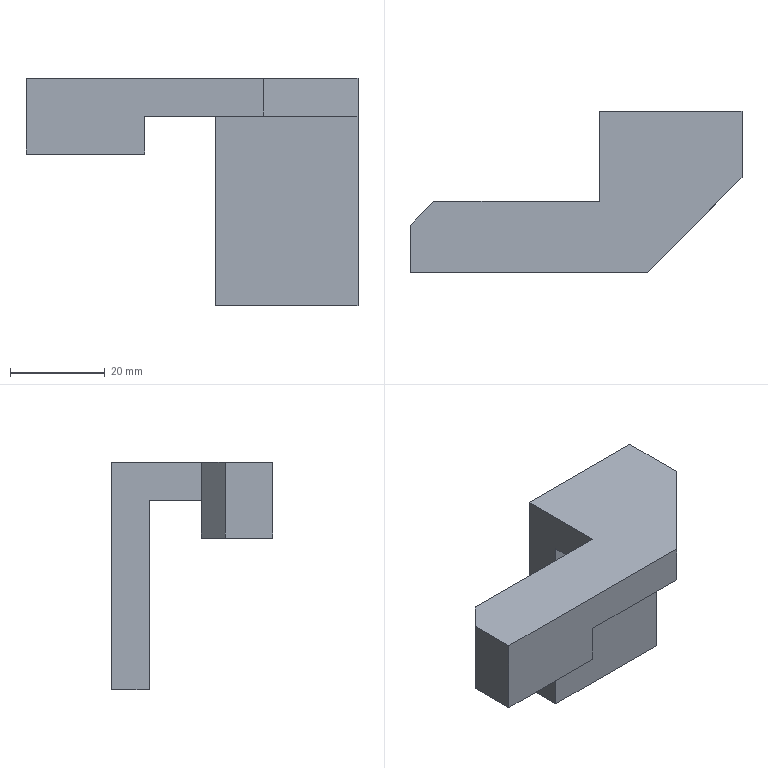Part | SolidWorks | features ICE 3, Chamfer 2, Extrusion 1 | 1 solid | 14 faces | box 70 x 34 x 48 mm | volume 23760 mm3 | plane 14
STEP:
#1=CARTESIAN_POINT('',(15.,-6.,20.));
#2=VERTEX_POINT('',#1);
#3=CARTESIAN_POINT('',(15.,0.,20.));
#4=VERTEX_POINT('',#3);
#5=CARTESIAN_POINT('',(15.,8.,20.));
#6=DIRECTION('',(0.,1.,0.));
#7=VECTOR('',#6,1000.);
#8=LINE('',#5,#7);
#9=EDGE_CURVE('',#2,#4,#8,.T.);
#10=ORIENTED_EDGE('',*,*,#9,.F.);
#11=CARTESIAN_POINT('',(-5.,-26.,20.));
#12=VERTEX_POINT('',#11);
#13=CARTESIAN_POINT('',(15.,-6.,20.));
#14=DIRECTION('',(-0.7071,-0.7071,0.));
#15=VECTOR('',#14,1000.);
#16=LINE('',#13,#15);
#17=EDGE_CURVE('',#2,#12,#16,.T.);
#18=ORIENTED_EDGE('',*,*,#17,.T.);
#19=CARTESIAN_POINT('',(-30.,-26.,20.));
#20=VERTEX_POINT('',#19);
#21=CARTESIAN_POINT('',(-15.,-26.,20.));
#22=DIRECTION('',(1.,0.,0.));
#23=VECTOR('',#22,1000.);
#24=LINE('',#21,#23);
#25=EDGE_CURVE('',#20,#12,#24,.T.);
#26=ORIENTED_EDGE('',*,*,#25,.F.);
#27=CARTESIAN_POINT('',(-30.,-11.,20.));
#28=VERTEX_POINT('',#27);
#29=CARTESIAN_POINT('',(-30.,-26.,20.));
#30=DIRECTION('',(0.,-1.,0.));
#31=VECTOR('',#30,1000.);
#32=LINE('',#29,#31);
#33=EDGE_CURVE('',#28,#20,#32,.T.);
#34=ORIENTED_EDGE('',*,*,#33,.F.);
#35=CARTESIAN_POINT('',(-15.,-11.,20.));
#36=VERTEX_POINT('',#35);
#37=CARTESIAN_POINT('',(-55.,-11.,20.));
#38=DIRECTION('',(1.,0.,0.));
#39=VECTOR('',#38,1000.);
#40=LINE('',#37,#39);
#41=EDGE_CURVE('',#28,#36,#40,.T.);
#42=ORIENTED_EDGE('',*,*,#41,.T.);
#43=CARTESIAN_POINT('',(-15.,0.,20.));
#44=VERTEX_POINT('',#43);
#45=CARTESIAN_POINT('',(-15.,8.,20.));
#46=DIRECTION('',(0.,-1.,0.));
#47=VECTOR('',#46,1000.);
#48=LINE('',#45,#47);
#49=EDGE_CURVE('',#44,#36,#48,.T.);
#50=ORIENTED_EDGE('',*,*,#49,.F.);
#51=CARTESIAN_POINT('',(-15.,0.,20.));
#52=DIRECTION('',(1.,0.,0.));
#53=VECTOR('',#52,1000.);
#54=LINE('',#51,#53);
#55=EDGE_CURVE('',#44,#4,#54,.T.);
#56=ORIENTED_EDGE('',*,*,#55,.T.);
#57=EDGE_LOOP('',(#10,#18,#26,#34,#42,#50,#56));
#58=FACE_OUTER_BOUND('',#57,.T.);
#59=CARTESIAN_POINT('',(0.,0.,20.));
#60=DIRECTION('',(0.,0.,1.));
#61=DIRECTION('',(1.,0.,0.));
#62=AXIS2_PLACEMENT_3D('',#59,#60,#61);
#63=PLANE('',#62);
#64=ADVANCED_FACE('',(#58),#63,.F.);
#65=CARTESIAN_POINT('',(-15.,-11.,28.));
#66=VERTEX_POINT('',#65);
#67=CARTESIAN_POINT('',(-15.,-11.,20.));
#68=DIRECTION('',(0.,0.,-1.));
#69=VECTOR('',#68,1000.);
#70=LINE('',#67,#69);
#71=EDGE_CURVE('',#66,#36,#70,.T.);
#72=ORIENTED_EDGE('',*,*,#71,.F.);
#73=CARTESIAN_POINT('',(-15.,8.,28.));
#74=VERTEX_POINT('',#73);
#75=CARTESIAN_POINT('',(-15.,8.,28.));
#76=DIRECTION('',(0.,-1.,0.));
#77=VECTOR('',#76,1000.);
#78=LINE('',#75,#77);
#79=EDGE_CURVE('',#74,#66,#78,.T.);
#80=ORIENTED_EDGE('',*,*,#79,.F.);
#81=CARTESIAN_POINT('',(-15.,8.,-20.));
#82=VERTEX_POINT('',#81);
#83=CARTESIAN_POINT('',(-15.,8.,-20.));
#84=DIRECTION('',(0.,0.,1.));
#85=VECTOR('',#84,1000.);
#86=LINE('',#83,#85);
#87=EDGE_CURVE('',#82,#74,#86,.T.);
#88=ORIENTED_EDGE('',*,*,#87,.F.);
#89=CARTESIAN_POINT('',(-15.,0.,-20.));
#90=VERTEX_POINT('',#89);
#91=CARTESIAN_POINT('',(-15.,8.,-20.));
#92=DIRECTION('',(0.,-1.,0.));
#93=VECTOR('',#92,1000.);
#94=LINE('',#91,#93);
#95=EDGE_CURVE('',#82,#90,#94,.T.);
#96=ORIENTED_EDGE('',*,*,#95,.T.);
#97=CARTESIAN_POINT('',(-15.,0.,-20.));
#98=DIRECTION('',(0.,0.,1.));
#99=VECTOR('',#98,1000.);
#100=LINE('',#97,#99);
#101=EDGE_CURVE('',#90,#44,#100,.T.);
#102=ORIENTED_EDGE('',*,*,#101,.T.);
#103=ORIENTED_EDGE('',*,*,#49,.T.);
#104=EDGE_LOOP('',(#72,#80,#88,#96,#102,#103));
#105=FACE_OUTER_BOUND('',#104,.T.);
#106=CARTESIAN_POINT('',(-15.,8.,-20.));
#107=DIRECTION('',(1.,0.,0.));
#108=DIRECTION('',(0.,0.,-1.));
#109=AXIS2_PLACEMENT_3D('',#106,#107,#108);
#110=PLANE('',#109);
#111=ADVANCED_FACE('',(#105),#110,.F.);
#112=CARTESIAN_POINT('',(15.,-6.,28.));
#113=VERTEX_POINT('',#112);
#114=CARTESIAN_POINT('',(15.,8.,28.));
#115=VERTEX_POINT('',#114);
#116=CARTESIAN_POINT('',(15.,8.,28.));
#117=DIRECTION('',(0.,1.,0.));
#118=VECTOR('',#117,1000.);
#119=LINE('',#116,#118);
#120=EDGE_CURVE('',#113,#115,#119,.T.);
#121=ORIENTED_EDGE('',*,*,#120,.F.);
#122=CARTESIAN_POINT('',(15.,-6.,-20.));
#123=DIRECTION('',(0.,0.,-1.));
#124=VECTOR('',#123,1000.);
#125=LINE('',#122,#124);
#126=EDGE_CURVE('',#113,#2,#125,.T.);
#127=ORIENTED_EDGE('',*,*,#126,.T.);
#128=ORIENTED_EDGE('',*,*,#9,.T.);
#129=CARTESIAN_POINT('',(15.,0.,-20.));
#130=VERTEX_POINT('',#129);
#131=CARTESIAN_POINT('',(15.,0.,-20.));
#132=DIRECTION('',(0.,0.,-1.));
#133=VECTOR('',#132,1000.);
#134=LINE('',#131,#133);
#135=EDGE_CURVE('',#4,#130,#134,.T.);
#136=ORIENTED_EDGE('',*,*,#135,.T.);
#137=CARTESIAN_POINT('',(15.,8.,-20.));
#138=VERTEX_POINT('',#137);
#139=CARTESIAN_POINT('',(15.,8.,-20.));
#140=DIRECTION('',(0.,-1.,0.));
#141=VECTOR('',#140,1000.);
#142=LINE('',#139,#141);
#143=EDGE_CURVE('',#138,#130,#142,.T.);
#144=ORIENTED_EDGE('',*,*,#143,.F.);
#145=CARTESIAN_POINT('',(15.,8.,-20.));
#146=DIRECTION('',(0.,0.,-1.));
#147=VECTOR('',#146,1000.);
#148=LINE('',#145,#147);
#149=EDGE_CURVE('',#115,#138,#148,.T.);
#150=ORIENTED_EDGE('',*,*,#149,.F.);
#151=EDGE_LOOP('',(#121,#127,#128,#136,#144,#150));
#152=FACE_OUTER_BOUND('',#151,.T.);
#153=CARTESIAN_POINT('',(15.,8.,-20.));
#154=DIRECTION('',(-1.,0.,0.));
#155=DIRECTION('',(0.,0.,1.));
#156=AXIS2_PLACEMENT_3D('',#153,#154,#155);
#157=PLANE('',#156);
#158=ADVANCED_FACE('',(#152),#157,.F.);
#159=CARTESIAN_POINT('',(-15.,0.,-20.));
#160=DIRECTION('',(-1.,0.,0.));
#161=VECTOR('',#160,1000.);
#162=LINE('',#159,#161);
#163=EDGE_CURVE('',#130,#90,#162,.T.);
#164=ORIENTED_EDGE('',*,*,#163,.T.);
#165=ORIENTED_EDGE('',*,*,#95,.F.);
#166=CARTESIAN_POINT('',(-15.,8.,-20.));
#167=DIRECTION('',(-1.,0.,0.));
#168=VECTOR('',#167,1000.);
#169=LINE('',#166,#168);
#170=EDGE_CURVE('',#138,#82,#169,.T.);
#171=ORIENTED_EDGE('',*,*,#170,.F.);
#172=ORIENTED_EDGE('',*,*,#143,.T.);
#173=EDGE_LOOP('',(#164,#165,#171,#172));
#174=FACE_OUTER_BOUND('',#173,.T.);
#175=CARTESIAN_POINT('',(-15.,8.,-20.));
#176=DIRECTION('',(0.,0.,1.));
#177=DIRECTION('',(1.,0.,0.));
#178=AXIS2_PLACEMENT_3D('',#175,#176,#177);
#179=PLANE('',#178);
#180=ADVANCED_FACE('',(#174),#179,.F.);
#181=ORIENTED_EDGE('',*,*,#87,.T.);
#182=CARTESIAN_POINT('',(-15.,8.,28.));
#183=DIRECTION('',(-1.,0.,0.));
#184=VECTOR('',#183,1000.);
#185=LINE('',#182,#184);
#186=EDGE_CURVE('',#115,#74,#185,.T.);
#187=ORIENTED_EDGE('',*,*,#186,.F.);
#188=ORIENTED_EDGE('',*,*,#149,.T.);
#189=ORIENTED_EDGE('',*,*,#170,.T.);
#190=EDGE_LOOP('',(#181,#187,#188,#189));
#191=FACE_OUTER_BOUND('',#190,.T.);
#192=CARTESIAN_POINT('',(0.,8.,0.));
#193=DIRECTION('',(0.,1.,0.));
#194=DIRECTION('',(0.,0.,1.));
#195=AXIS2_PLACEMENT_3D('',#192,#193,#194);
#196=PLANE('',#195);
#197=ADVANCED_FACE('',(#191),#196,.T.);
#198=ORIENTED_EDGE('',*,*,#101,.F.);
#199=ORIENTED_EDGE('',*,*,#163,.F.);
#200=ORIENTED_EDGE('',*,*,#135,.F.);
#201=ORIENTED_EDGE('',*,*,#55,.F.);
#202=EDGE_LOOP('',(#198,#199,#200,#201));
#203=FACE_OUTER_BOUND('',#202,.T.);
#204=CARTESIAN_POINT('',(0.,0.,0.));
#205=DIRECTION('',(0.,1.,0.));
#206=DIRECTION('',(0.,0.,1.));
#207=AXIS2_PLACEMENT_3D('',#204,#205,#206);
#208=PLANE('',#207);
#209=ADVANCED_FACE('',(#203),#208,.F.);
#210=ORIENTED_EDGE('',*,*,#25,.T.);
#211=CARTESIAN_POINT('',(-5.,-26.,28.));
#212=VERTEX_POINT('',#211);
#213=CARTESIAN_POINT('',(-5.,-26.,28.));
#214=DIRECTION('',(0.,0.,1.));
#215=VECTOR('',#214,1000.);
#216=LINE('',#213,#215);
#217=EDGE_CURVE('',#12,#212,#216,.T.);
#218=ORIENTED_EDGE('',*,*,#217,.T.);
#219=CARTESIAN_POINT('',(-55.,-26.,28.));
#220=VERTEX_POINT('',#219);
#221=CARTESIAN_POINT('',(-15.,-26.,28.));
#222=DIRECTION('',(1.,0.,0.));
#223=VECTOR('',#222,1000.);
#224=LINE('',#221,#223);
#225=EDGE_CURVE('',#220,#212,#224,.T.);
#226=ORIENTED_EDGE('',*,*,#225,.F.);
#227=CARTESIAN_POINT('',(-55.,-26.,12.));
#228=VERTEX_POINT('',#227);
#229=CARTESIAN_POINT('',(-55.,-26.,20.));
#230=DIRECTION('',(0.,0.,1.));
#231=VECTOR('',#230,1000.);
#232=LINE('',#229,#231);
#233=EDGE_CURVE('',#228,#220,#232,.T.);
#234=ORIENTED_EDGE('',*,*,#233,.F.);
#235=CARTESIAN_POINT('',(-30.,-26.,12.));
#236=VERTEX_POINT('',#235);
#237=CARTESIAN_POINT('',(-55.,-26.,12.));
#238=DIRECTION('',(-1.,0.,0.));
#239=VECTOR('',#238,1000.);
#240=LINE('',#237,#239);
#241=EDGE_CURVE('',#236,#228,#240,.T.);
#242=ORIENTED_EDGE('',*,*,#241,.F.);
#243=CARTESIAN_POINT('',(-30.,-26.,12.));
#244=DIRECTION('',(0.,0.,1.));
#245=VECTOR('',#244,1000.);
#246=LINE('',#243,#245);
#247=EDGE_CURVE('',#236,#20,#246,.T.);
#248=ORIENTED_EDGE('',*,*,#247,.T.);
#249=EDGE_LOOP('',(#210,#218,#226,#234,#242,#248));
#250=FACE_OUTER_BOUND('',#249,.T.);
#251=CARTESIAN_POINT('',(-15.,-26.,28.));
#252=DIRECTION('',(0.,1.,0.));
#253=DIRECTION('',(-1.,0.,0.));
#254=AXIS2_PLACEMENT_3D('',#251,#252,#253);
#255=PLANE('',#254);
#256=ADVANCED_FACE('',(#250),#255,.F.);
#257=ORIENTED_EDGE('',*,*,#225,.T.);
#258=CARTESIAN_POINT('',(10.5,-10.5,28.));
#259=DIRECTION('',(0.7071,0.7071,0.));
#260=VECTOR('',#259,1000.);
#261=LINE('',#258,#260);
#262=EDGE_CURVE('',#212,#113,#261,.T.);
#263=ORIENTED_EDGE('',*,*,#262,.T.);
#264=ORIENTED_EDGE('',*,*,#120,.T.);
#265=ORIENTED_EDGE('',*,*,#186,.T.);
#266=ORIENTED_EDGE('',*,*,#79,.T.);
#267=CARTESIAN_POINT('',(-50.,-11.,28.));
#268=VERTEX_POINT('',#267);
#269=CARTESIAN_POINT('',(-55.,-11.,28.));
#270=DIRECTION('',(1.,0.,0.));
#271=VECTOR('',#270,1000.);
#272=LINE('',#269,#271);
#273=EDGE_CURVE('',#268,#66,#272,.T.);
#274=ORIENTED_EDGE('',*,*,#273,.F.);
#275=CARTESIAN_POINT('',(-55.,-16.,28.));
#276=VERTEX_POINT('',#275);
#277=CARTESIAN_POINT('',(-19.5,19.5,28.));
#278=DIRECTION('',(-0.7071,-0.7071,0.));
#279=VECTOR('',#278,1000.);
#280=LINE('',#277,#279);
#281=EDGE_CURVE('',#268,#276,#280,.T.);
#282=ORIENTED_EDGE('',*,*,#281,.T.);
#283=CARTESIAN_POINT('',(-55.,-26.,28.));
#284=DIRECTION('',(0.,1.,0.));
#285=VECTOR('',#284,1000.);
#286=LINE('',#283,#285);
#287=EDGE_CURVE('',#220,#276,#286,.T.);
#288=ORIENTED_EDGE('',*,*,#287,.F.);
#289=EDGE_LOOP('',(#257,#263,#264,#265,#266,#274,#282,#288));
#290=FACE_OUTER_BOUND('',#289,.T.);
#291=CARTESIAN_POINT('',(0.,0.,28.));
#292=DIRECTION('',(0.,0.,1.));
#293=DIRECTION('',(1.,0.,0.));
#294=AXIS2_PLACEMENT_3D('',#291,#292,#293);
#295=PLANE('',#294);
#296=ADVANCED_FACE('',(#290),#295,.T.);
#297=ORIENTED_EDGE('',*,*,#41,.F.);
#298=CARTESIAN_POINT('',(-30.,-11.,12.));
#299=VERTEX_POINT('',#298);
#300=CARTESIAN_POINT('',(-30.,-11.,12.));
#301=DIRECTION('',(0.,0.,1.));
#302=VECTOR('',#301,1000.);
#303=LINE('',#300,#302);
#304=EDGE_CURVE('',#299,#28,#303,.T.);
#305=ORIENTED_EDGE('',*,*,#304,.F.);
#306=CARTESIAN_POINT('',(-50.,-11.,12.));
#307=VERTEX_POINT('',#306);
#308=CARTESIAN_POINT('',(-30.,-11.,12.));
#309=DIRECTION('',(1.,0.,0.));
#310=VECTOR('',#309,1000.);
#311=LINE('',#308,#310);
#312=EDGE_CURVE('',#307,#299,#311,.T.);
#313=ORIENTED_EDGE('',*,*,#312,.F.);
#314=CARTESIAN_POINT('',(-50.,-11.,20.));
#315=DIRECTION('',(0.,0.,1.));
#316=VECTOR('',#315,1000.);
#317=LINE('',#314,#316);
#318=EDGE_CURVE('',#307,#268,#317,.T.);
#319=ORIENTED_EDGE('',*,*,#318,.T.);
#320=ORIENTED_EDGE('',*,*,#273,.T.);
#321=ORIENTED_EDGE('',*,*,#71,.T.);
#322=EDGE_LOOP('',(#297,#305,#313,#319,#320,#321));
#323=FACE_OUTER_BOUND('',#322,.T.);
#324=CARTESIAN_POINT('',(-55.,-11.,20.));
#325=DIRECTION('',(0.,-1.,0.));
#326=DIRECTION('',(0.,0.,-1.));
#327=AXIS2_PLACEMENT_3D('',#324,#325,#326);
#328=PLANE('',#327);
#329=ADVANCED_FACE('',(#323),#328,.F.);
#330=ORIENTED_EDGE('',*,*,#287,.T.);
#331=CARTESIAN_POINT('',(-55.,-16.,12.));
#332=VERTEX_POINT('',#331);
#333=CARTESIAN_POINT('',(-55.,-16.,0.));
#334=DIRECTION('',(0.,0.,-1.));
#335=VECTOR('',#334,1000.);
#336=LINE('',#333,#335);
#337=EDGE_CURVE('',#276,#332,#336,.T.);
#338=ORIENTED_EDGE('',*,*,#337,.T.);
#339=CARTESIAN_POINT('',(-55.,-16.,12.));
#340=DIRECTION('',(0.,1.,0.));
#341=VECTOR('',#340,1000.);
#342=LINE('',#339,#341);
#343=EDGE_CURVE('',#228,#332,#342,.T.);
#344=ORIENTED_EDGE('',*,*,#343,.F.);
#345=ORIENTED_EDGE('',*,*,#233,.T.);
#346=EDGE_LOOP('',(#330,#338,#344,#345));
#347=FACE_OUTER_BOUND('',#346,.T.);
#348=CARTESIAN_POINT('',(-55.,0.,0.));
#349=DIRECTION('',(1.,0.,0.));
#350=DIRECTION('',(0.,0.,-1.));
#351=AXIS2_PLACEMENT_3D('',#348,#349,#350);
#352=PLANE('',#351);
#353=ADVANCED_FACE('',(#347),#352,.F.);
#354=ORIENTED_EDGE('',*,*,#281,.F.);
#355=ORIENTED_EDGE('',*,*,#318,.F.);
#356=CARTESIAN_POINT('',(-50.,-11.,12.));
#357=DIRECTION('',(0.7071,0.7071,0.));
#358=VECTOR('',#357,1000.);
#359=LINE('',#356,#358);
#360=EDGE_CURVE('',#332,#307,#359,.T.);
#361=ORIENTED_EDGE('',*,*,#360,.F.);
#362=ORIENTED_EDGE('',*,*,#337,.F.);
#363=EDGE_LOOP('',(#354,#355,#361,#362));
#364=FACE_OUTER_BOUND('',#363,.T.);
#365=CARTESIAN_POINT('',(-55.,-16.,0.));
#366=DIRECTION('',(0.7071,-0.7071,0.));
#367=DIRECTION('',(0.,0.,-1.));
#368=AXIS2_PLACEMENT_3D('',#365,#366,#367);
#369=PLANE('',#368);
#370=ADVANCED_FACE('',(#364),#369,.F.);
#371=ORIENTED_EDGE('',*,*,#33,.T.);
#372=ORIENTED_EDGE('',*,*,#247,.F.);
#373=CARTESIAN_POINT('',(-30.,-26.,12.));
#374=DIRECTION('',(0.,-1.,0.));
#375=VECTOR('',#374,1000.);
#376=LINE('',#373,#375);
#377=EDGE_CURVE('',#299,#236,#376,.T.);
#378=ORIENTED_EDGE('',*,*,#377,.F.);
#379=ORIENTED_EDGE('',*,*,#304,.T.);
#380=EDGE_LOOP('',(#371,#372,#378,#379));
#381=FACE_OUTER_BOUND('',#380,.T.);
#382=CARTESIAN_POINT('',(-30.,-26.,12.));
#383=DIRECTION('',(-1.,0.,0.));
#384=DIRECTION('',(0.,-1.,0.));
#385=AXIS2_PLACEMENT_3D('',#382,#383,#384);
#386=PLANE('',#385);
#387=ADVANCED_FACE('',(#381),#386,.F.);
#388=ORIENTED_EDGE('',*,*,#377,.T.);
#389=ORIENTED_EDGE('',*,*,#241,.T.);
#390=ORIENTED_EDGE('',*,*,#343,.T.);
#391=ORIENTED_EDGE('',*,*,#360,.T.);
#392=ORIENTED_EDGE('',*,*,#312,.T.);
#393=EDGE_LOOP('',(#388,#389,#390,#391,#392));
#394=FACE_OUTER_BOUND('',#393,.T.);
#395=CARTESIAN_POINT('',(0.,0.,12.));
#396=DIRECTION('',(0.,0.,1.));
#397=DIRECTION('',(1.,0.,0.));
#398=AXIS2_PLACEMENT_3D('',#395,#396,#397);
#399=PLANE('',#398);
#400=ADVANCED_FACE('',(#394),#399,.F.);
#401=ORIENTED_EDGE('',*,*,#262,.F.);
#402=ORIENTED_EDGE('',*,*,#217,.F.);
#403=ORIENTED_EDGE('',*,*,#17,.F.);
#404=ORIENTED_EDGE('',*,*,#126,.F.);
#405=EDGE_LOOP('',(#401,#402,#403,#404));
#406=FACE_OUTER_BOUND('',#405,.T.);
#407=CARTESIAN_POINT('',(15.,-6.,-20.));
#408=DIRECTION('',(-0.7071,0.7071,0.));
#409=DIRECTION('',(0.,0.,-1.));
#410=AXIS2_PLACEMENT_3D('',#407,#408,#409);
#411=PLANE('',#410);
#412=ADVANCED_FACE('',(#406),#411,.F.);
#413=CLOSED_SHELL('',(#64,#111,#158,#180,#197,#209,#256,#296,#329,#353,#370,#387,#400,#412));
#414=MANIFOLD_SOLID_BREP('',#413);
#415=CARTESIAN_POINT('',(0.,0.,0.));
#416=DIRECTION('',(0.,0.,1.));
#417=DIRECTION('',(1.,0.,0.));
#418=AXIS2_PLACEMENT_3D('',#415,#416,#417);
#419=(LENGTH_UNIT()NAMED_UNIT(*)SI_UNIT(.MILLI.,.METRE.));
#420=UNCERTAINTY_MEASURE_WITH_UNIT(LENGTH_MEASURE(0.00001),#419,'','');
#421=(NAMED_UNIT(*)PLANE_ANGLE_UNIT()SI_UNIT($,.RADIAN.));
#422=(NAMED_UNIT(*)SI_UNIT($,.STERADIAN.)SOLID_ANGLE_UNIT());
#423=(GEOMETRIC_REPRESENTATION_CONTEXT(3)GLOBAL_UNCERTAINTY_ASSIGNED_CONTEXT((#420))GLOBAL_UNIT_ASSIGNED_CONTEXT((#419,#421,#422))REPRESENTATION_CONTEXT('',''));
#424=ADVANCED_BREP_SHAPE_REPRESENTATION('',(#414,#418),#423);